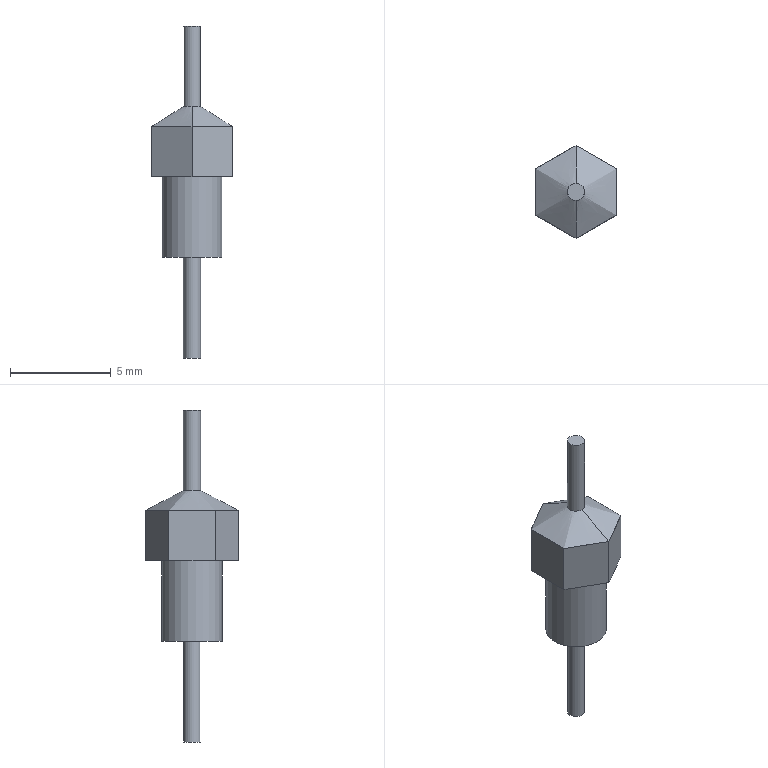Part | STEP file | Feed through capacitor M3 | 3 solids | 19 faces | box 4 x 4.619 x 16.5 mm | volume 73.685 mm3 | plane 14 | cylinder 3 | spline 2 | commonest cylinder face diameters 0.85 x2 3 x1